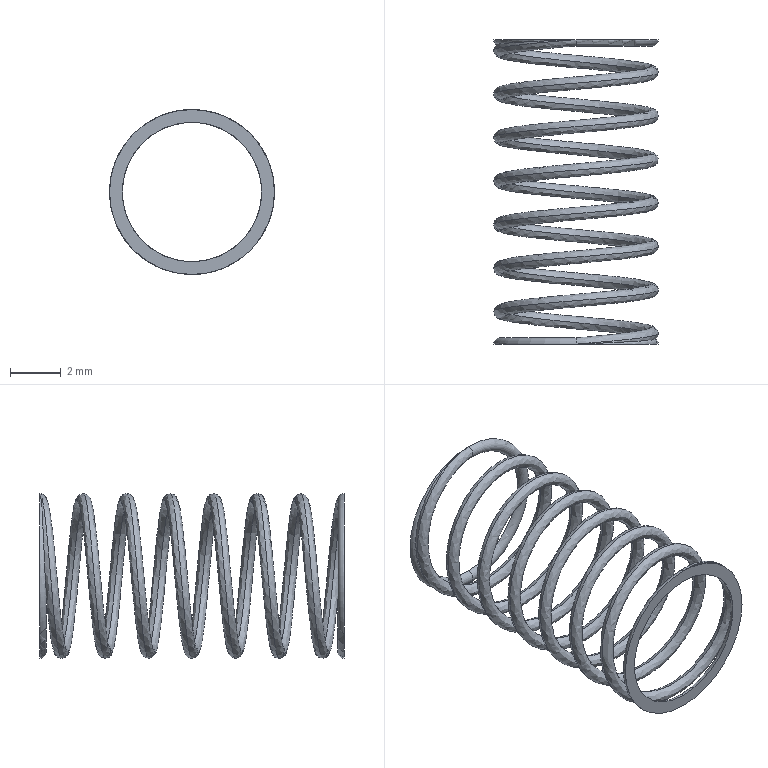Part | NX | features BREP 1 | 1 solid | 8 faces | box 6.5 x 12 x 6.5 mm | volume 28.674 mm3 | torus 4 | spline 2 | plane 2